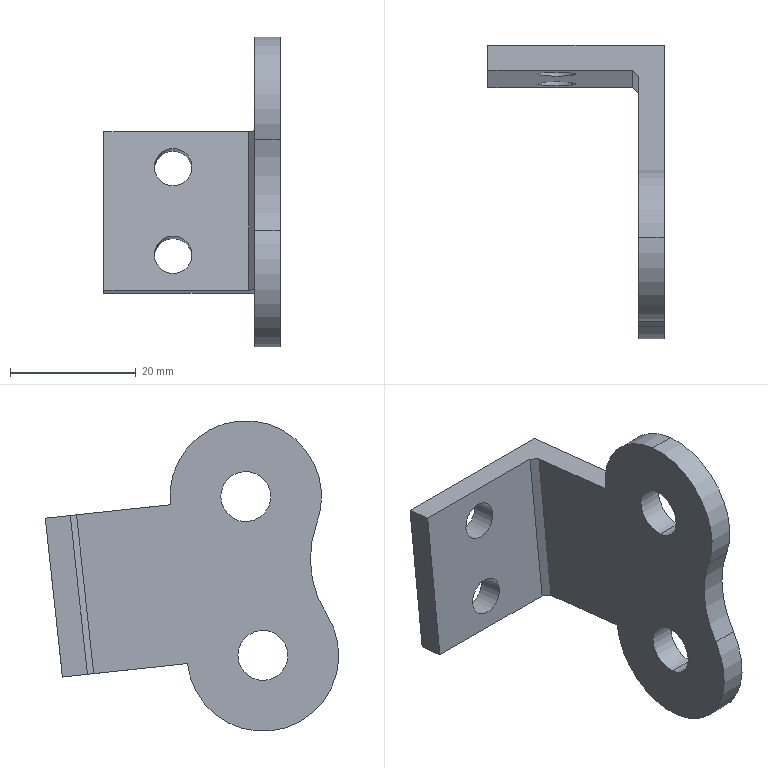Part | STEP file | Cut-Extrude 2-4 | 1 solid | 21 faces | box 28 x 46.671 x 49.383 mm | volume 7981 mm3 | cylinder 13 | plane 8 | commonest cylinder face diameters 6 x4 7.94 x4 24.13 x4 32.482 x1
STEP:
#1=CARTESIAN_POINT('',(303.74,-1270.259,3580.538));
#2=VERTEX_POINT('',#1);
#3=CARTESIAN_POINT('',(303.74,-1259.559,3567.248));
#4=VERTEX_POINT('',#3);
#5=CARTESIAN_POINT('',(303.74,-1271.554,3568.543));
#6=DIRECTION('',(-1.,0.,0.));
#7=DIRECTION('',(0.,0.1073,0.9942));
#8=AXIS2_PLACEMENT_3D('',#5,#6,#7);
#9=CIRCLE('',#8,12.065);
#10=EDGE_CURVE('',#2,#4,#9,.T.);
#11=ORIENTED_EDGE('',*,*,#10,.F.);
#12=CARTESIAN_POINT('',(307.74,-1270.259,3580.538));
#13=VERTEX_POINT('',#12);
#14=CARTESIAN_POINT('',(303.74,-1270.259,3580.538));
#15=DIRECTION('',(1.,0.,0.));
#16=VECTOR('',#15,1000.);
#17=LINE('',#14,#16);
#18=EDGE_CURVE('',#2,#13,#17,.T.);
#19=ORIENTED_EDGE('',*,*,#18,.T.);
#20=CARTESIAN_POINT('',(307.74,-1259.559,3567.248));
#21=VERTEX_POINT('',#20);
#22=CARTESIAN_POINT('',(307.74,-1271.554,3568.543));
#23=DIRECTION('',(-1.,0.,0.));
#24=DIRECTION('',(0.,0.1073,0.9942));
#25=AXIS2_PLACEMENT_3D('',#22,#23,#24);
#26=CIRCLE('',#25,12.065);
#27=EDGE_CURVE('',#13,#21,#26,.T.);
#28=ORIENTED_EDGE('',*,*,#27,.T.);
#29=CARTESIAN_POINT('',(303.74,-1259.559,3567.248));
#30=DIRECTION('',(1.,0.,0.));
#31=VECTOR('',#30,1000.);
#32=LINE('',#29,#31);
#33=EDGE_CURVE('',#4,#21,#32,.T.);
#34=ORIENTED_EDGE('',*,*,#33,.F.);
#35=EDGE_LOOP('',(#11,#19,#28,#34));
#36=FACE_OUTER_BOUND('',#35,.T.);
#37=CARTESIAN_POINT('',(303.74,-1271.554,3568.543));
#38=DIRECTION('',(1.,0.,0.));
#39=DIRECTION('',(0.,0.1073,0.9942));
#40=AXIS2_PLACEMENT_3D('',#37,#38,#39);
#41=CYLINDRICAL_SURFACE('',#40,12.065);
#42=ADVANCED_FACE('',(#36),#41,.T.);
#43=CARTESIAN_POINT('',(287.74,-1245.766,3545.944));
#44=VERTEX_POINT('',#43);
#45=CARTESIAN_POINT('',(293.74,-1245.766,3545.944));
#46=VERTEX_POINT('',#45);
#47=CARTESIAN_POINT('',(290.74,-1245.766,3545.944));
#48=DIRECTION('',(0.,-0.9942,0.1073));
#49=DIRECTION('',(1.,0.,0.));
#50=AXIS2_PLACEMENT_3D('',#47,#48,#49);
#51=CIRCLE('',#50,3.);
#52=EDGE_CURVE('',#44,#46,#51,.T.);
#53=ORIENTED_EDGE('',*,*,#52,.T.);
#54=CARTESIAN_POINT('',(293.74,-1241.789,3545.515));
#55=VERTEX_POINT('',#54);
#56=CARTESIAN_POINT('',(293.74,-1285.664,3550.251));
#57=DIRECTION('',(0.,0.9942,-0.1073));
#58=VECTOR('',#57,1000.);
#59=LINE('',#56,#58);
#60=EDGE_CURVE('',#46,#55,#59,.T.);
#61=ORIENTED_EDGE('',*,*,#60,.T.);
#62=CARTESIAN_POINT('',(287.74,-1241.789,3545.515));
#63=VERTEX_POINT('',#62);
#64=CARTESIAN_POINT('',(290.74,-1241.789,3545.515));
#65=DIRECTION('',(0.,0.9942,-0.1073));
#66=DIRECTION('',(-1.,0.,0.));
#67=AXIS2_PLACEMENT_3D('',#64,#65,#66);
#68=CIRCLE('',#67,3.);
#69=EDGE_CURVE('',#55,#63,#68,.T.);
#70=ORIENTED_EDGE('',*,*,#69,.T.);
#71=CARTESIAN_POINT('',(287.74,-1285.664,3550.251));
#72=DIRECTION('',(0.,0.9942,-0.1073));
#73=VECTOR('',#72,1000.);
#74=LINE('',#71,#73);
#75=EDGE_CURVE('',#44,#63,#74,.T.);
#76=ORIENTED_EDGE('',*,*,#75,.F.);
#77=EDGE_LOOP('',(#53,#61,#70,#76));
#78=FACE_OUTER_BOUND('',#77,.T.);
#79=CARTESIAN_POINT('',(290.74,-1285.664,3550.251));
#80=DIRECTION('',(0.,0.9942,-0.1073));
#81=DIRECTION('',(1.,0.,0.));
#82=AXIS2_PLACEMENT_3D('',#79,#80,#81);
#83=CYLINDRICAL_SURFACE('',#82,3.);
#84=ADVANCED_FACE('',(#78),#83,.F.);
#85=CARTESIAN_POINT('',(287.74,-1244.263,3559.863));
#86=VERTEX_POINT('',#85);
#87=CARTESIAN_POINT('',(293.74,-1244.263,3559.863));
#88=VERTEX_POINT('',#87);
#89=CARTESIAN_POINT('',(290.74,-1244.263,3559.863));
#90=DIRECTION('',(0.,-0.9942,0.1073));
#91=DIRECTION('',(1.,0.,0.));
#92=AXIS2_PLACEMENT_3D('',#89,#90,#91);
#93=CIRCLE('',#92,3.);
#94=EDGE_CURVE('',#86,#88,#93,.T.);
#95=ORIENTED_EDGE('',*,*,#94,.T.);
#96=CARTESIAN_POINT('',(293.74,-1240.286,3559.434));
#97=VERTEX_POINT('',#96);
#98=CARTESIAN_POINT('',(293.74,-1284.161,3564.171));
#99=DIRECTION('',(0.,0.9942,-0.1073));
#100=VECTOR('',#99,1000.);
#101=LINE('',#98,#100);
#102=EDGE_CURVE('',#88,#97,#101,.T.);
#103=ORIENTED_EDGE('',*,*,#102,.T.);
#104=CARTESIAN_POINT('',(287.74,-1240.286,3559.434));
#105=VERTEX_POINT('',#104);
#106=CARTESIAN_POINT('',(290.74,-1240.286,3559.434));
#107=DIRECTION('',(0.,0.9942,-0.1073));
#108=DIRECTION('',(1.,0.,0.));
#109=AXIS2_PLACEMENT_3D('',#106,#107,#108);
#110=CIRCLE('',#109,3.);
#111=EDGE_CURVE('',#97,#105,#110,.T.);
#112=ORIENTED_EDGE('',*,*,#111,.T.);
#113=CARTESIAN_POINT('',(287.74,-1284.161,3564.171));
#114=DIRECTION('',(0.,0.9942,-0.1073));
#115=VECTOR('',#114,1000.);
#116=LINE('',#113,#115);
#117=EDGE_CURVE('',#86,#105,#116,.T.);
#118=ORIENTED_EDGE('',*,*,#117,.F.);
#119=EDGE_LOOP('',(#95,#103,#112,#118));
#120=FACE_OUTER_BOUND('',#119,.T.);
#121=CARTESIAN_POINT('',(290.74,-1284.161,3564.171));
#122=DIRECTION('',(0.,0.9942,-0.1073));
#123=DIRECTION('',(1.,0.,0.));
#124=AXIS2_PLACEMENT_3D('',#121,#122,#123);
#125=CYLINDRICAL_SURFACE('',#124,3.);
#126=ADVANCED_FACE('',(#120),#125,.F.);
#127=CARTESIAN_POINT('',(303.74,-1271.128,3572.49));
#128=VERTEX_POINT('',#127);
#129=CARTESIAN_POINT('',(303.74,-1271.98,3564.596));
#130=VERTEX_POINT('',#129);
#131=CARTESIAN_POINT('',(303.74,-1271.554,3568.543));
#132=DIRECTION('',(1.,0.,0.));
#133=DIRECTION('',(0.,-0.1073,-0.9942));
#134=AXIS2_PLACEMENT_3D('',#131,#132,#133);
#135=CIRCLE('',#134,3.97);
#136=EDGE_CURVE('',#128,#130,#135,.T.);
#137=ORIENTED_EDGE('',*,*,#136,.F.);
#138=CARTESIAN_POINT('',(307.74,-1271.128,3572.49));
#139=VERTEX_POINT('',#138);
#140=CARTESIAN_POINT('',(303.74,-1271.128,3572.49));
#141=DIRECTION('',(-1.,0.,0.));
#142=VECTOR('',#141,1000.);
#143=LINE('',#140,#142);
#144=EDGE_CURVE('',#139,#128,#143,.T.);
#145=ORIENTED_EDGE('',*,*,#144,.F.);
#146=CARTESIAN_POINT('',(307.74,-1271.98,3564.596));
#147=VERTEX_POINT('',#146);
#148=CARTESIAN_POINT('',(307.74,-1271.554,3568.543));
#149=DIRECTION('',(1.,0.,0.));
#150=DIRECTION('',(0.,-0.1073,-0.9942));
#151=AXIS2_PLACEMENT_3D('',#148,#149,#150);
#152=CIRCLE('',#151,3.97);
#153=EDGE_CURVE('',#139,#147,#152,.T.);
#154=ORIENTED_EDGE('',*,*,#153,.T.);
#155=CARTESIAN_POINT('',(303.74,-1271.98,3564.596));
#156=DIRECTION('',(-1.,0.,0.));
#157=VECTOR('',#156,1000.);
#158=LINE('',#155,#157);
#159=EDGE_CURVE('',#147,#130,#158,.T.);
#160=ORIENTED_EDGE('',*,*,#159,.T.);
#161=EDGE_LOOP('',(#137,#145,#154,#160));
#162=FACE_OUTER_BOUND('',#161,.T.);
#163=CARTESIAN_POINT('',(303.74,-1271.554,3568.543));
#164=DIRECTION('',(1.,0.,0.));
#165=DIRECTION('',(0.,0.1073,0.9942));
#166=AXIS2_PLACEMENT_3D('',#163,#164,#165);
#167=CYLINDRICAL_SURFACE('',#166,3.97);
#168=ADVANCED_FACE('',(#162),#167,.F.);
#169=CARTESIAN_POINT('',(303.74,-1273.855,3547.236));
#170=VERTEX_POINT('',#169);
#171=CARTESIAN_POINT('',(303.74,-1274.707,3539.342));
#172=VERTEX_POINT('',#171);
#173=CARTESIAN_POINT('',(303.74,-1274.281,3543.289));
#174=DIRECTION('',(1.,0.,0.));
#175=DIRECTION('',(0.,0.1073,0.9942));
#176=AXIS2_PLACEMENT_3D('',#173,#174,#175);
#177=CIRCLE('',#176,3.97);
#178=EDGE_CURVE('',#170,#172,#177,.T.);
#179=ORIENTED_EDGE('',*,*,#178,.F.);
#180=CARTESIAN_POINT('',(307.74,-1273.855,3547.236));
#181=VERTEX_POINT('',#180);
#182=CARTESIAN_POINT('',(303.74,-1273.855,3547.236));
#183=DIRECTION('',(-1.,0.,0.));
#184=VECTOR('',#183,1000.);
#185=LINE('',#182,#184);
#186=EDGE_CURVE('',#181,#170,#185,.T.);
#187=ORIENTED_EDGE('',*,*,#186,.F.);
#188=CARTESIAN_POINT('',(307.74,-1274.707,3539.342));
#189=VERTEX_POINT('',#188);
#190=CARTESIAN_POINT('',(307.74,-1274.281,3543.289));
#191=DIRECTION('',(1.,0.,0.));
#192=DIRECTION('',(0.,0.1073,0.9942));
#193=AXIS2_PLACEMENT_3D('',#190,#191,#192);
#194=CIRCLE('',#193,3.97);
#195=EDGE_CURVE('',#181,#189,#194,.T.);
#196=ORIENTED_EDGE('',*,*,#195,.T.);
#197=CARTESIAN_POINT('',(303.74,-1274.707,3539.342));
#198=DIRECTION('',(-1.,0.,0.));
#199=VECTOR('',#198,1000.);
#200=LINE('',#197,#199);
#201=EDGE_CURVE('',#189,#172,#200,.T.);
#202=ORIENTED_EDGE('',*,*,#201,.T.);
#203=EDGE_LOOP('',(#179,#187,#196,#202));
#204=FACE_OUTER_BOUND('',#203,.T.);
#205=CARTESIAN_POINT('',(303.74,-1274.281,3543.289));
#206=DIRECTION('',(1.,0.,0.));
#207=DIRECTION('',(0.,0.1073,0.9942));
#208=AXIS2_PLACEMENT_3D('',#205,#206,#207);
#209=CYLINDRICAL_SURFACE('',#208,3.97);
#210=ADVANCED_FACE('',(#204),#209,.F.);
#211=CARTESIAN_POINT('',(303.74,-1275.576,3531.294));
#212=VERTEX_POINT('',#211);
#213=CARTESIAN_POINT('',(303.74,-1284.42,3549.829));
#214=VERTEX_POINT('',#213);
#215=CARTESIAN_POINT('',(303.74,-1274.281,3543.289));
#216=DIRECTION('',(-1.,0.,0.));
#217=DIRECTION('',(0.,0.1073,0.9942));
#218=AXIS2_PLACEMENT_3D('',#215,#216,#217);
#219=CIRCLE('',#218,12.065);
#220=EDGE_CURVE('',#212,#214,#219,.T.);
#221=ORIENTED_EDGE('',*,*,#220,.F.);
#222=CARTESIAN_POINT('',(307.74,-1275.576,3531.294));
#223=VERTEX_POINT('',#222);
#224=CARTESIAN_POINT('',(303.74,-1275.576,3531.294));
#225=DIRECTION('',(1.,0.,0.));
#226=VECTOR('',#225,1000.);
#227=LINE('',#224,#226);
#228=EDGE_CURVE('',#212,#223,#227,.T.);
#229=ORIENTED_EDGE('',*,*,#228,.T.);
#230=CARTESIAN_POINT('',(307.74,-1284.42,3549.829));
#231=VERTEX_POINT('',#230);
#232=CARTESIAN_POINT('',(307.74,-1274.281,3543.289));
#233=DIRECTION('',(-1.,0.,0.));
#234=DIRECTION('',(0.,0.1073,0.9942));
#235=AXIS2_PLACEMENT_3D('',#232,#233,#234);
#236=CIRCLE('',#235,12.065);
#237=EDGE_CURVE('',#223,#231,#236,.T.);
#238=ORIENTED_EDGE('',*,*,#237,.T.);
#239=CARTESIAN_POINT('',(303.74,-1284.42,3549.829));
#240=DIRECTION('',(1.,0.,0.));
#241=VECTOR('',#240,1000.);
#242=LINE('',#239,#241);
#243=EDGE_CURVE('',#214,#231,#242,.T.);
#244=ORIENTED_EDGE('',*,*,#243,.F.);
#245=EDGE_LOOP('',(#221,#229,#238,#244));
#246=FACE_OUTER_BOUND('',#245,.T.);
#247=CARTESIAN_POINT('',(303.74,-1274.281,3543.289));
#248=DIRECTION('',(1.,0.,0.));
#249=DIRECTION('',(0.,0.1073,0.9942));
#250=AXIS2_PLACEMENT_3D('',#247,#248,#249);
#251=CYLINDRICAL_SURFACE('',#250,12.065);
#252=ADVANCED_FACE('',(#246),#251,.T.);
#253=CARTESIAN_POINT('',(303.74,-1271.554,3568.543));
#254=DIRECTION('',(1.,0.,0.));
#255=DIRECTION('',(0.,-0.1073,-0.9942));
#256=AXIS2_PLACEMENT_3D('',#253,#254,#255);
#257=CIRCLE('',#256,3.97);
#258=EDGE_CURVE('',#130,#128,#257,.T.);
#259=ORIENTED_EDGE('',*,*,#258,.T.);
#260=ORIENTED_EDGE('',*,*,#136,.T.);
#261=EDGE_LOOP('',(#259,#260));
#262=FACE_BOUND('',#261,.T.);
#263=CARTESIAN_POINT('',(303.74,-1274.281,3543.289));
#264=DIRECTION('',(1.,0.,0.));
#265=DIRECTION('',(0.,0.1073,0.9942));
#266=AXIS2_PLACEMENT_3D('',#263,#264,#265);
#267=CIRCLE('',#266,3.97);
#268=EDGE_CURVE('',#172,#170,#267,.T.);
#269=ORIENTED_EDGE('',*,*,#268,.T.);
#270=ORIENTED_EDGE('',*,*,#178,.T.);
#271=EDGE_LOOP('',(#269,#270));
#272=FACE_BOUND('',#271,.T.);
#273=CARTESIAN_POINT('',(303.74,-1244.646,3565.637));
#274=VERTEX_POINT('',#273);
#275=CARTESIAN_POINT('',(303.74,-1239.674,3565.101));
#276=DIRECTION('',(0.,0.9942,-0.1073));
#277=VECTOR('',#276,1000.);
#278=LINE('',#275,#277);
#279=EDGE_CURVE('',#4,#274,#278,.T.);
#280=ORIENTED_EDGE('',*,*,#279,.T.);
#281=CARTESIAN_POINT('',(303.74,-1247.372,3540.384));
#282=VERTEX_POINT('',#281);
#283=CARTESIAN_POINT('',(303.74,-1247.372,3540.384));
#284=DIRECTION('',(0.,-0.1073,-0.9942));
#285=VECTOR('',#284,1000.);
#286=LINE('',#283,#285);
#287=EDGE_CURVE('',#274,#282,#286,.T.);
#288=ORIENTED_EDGE('',*,*,#287,.T.);
#289=CARTESIAN_POINT('',(303.74,-1262.285,3541.994));
#290=VERTEX_POINT('',#289);
#291=CARTESIAN_POINT('',(303.74,-1262.285,3541.994));
#292=DIRECTION('',(0.,-0.9942,0.1073));
#293=VECTOR('',#292,1000.);
#294=LINE('',#291,#293);
#295=EDGE_CURVE('',#282,#290,#294,.T.);
#296=ORIENTED_EDGE('',*,*,#295,.T.);
#297=CARTESIAN_POINT('',(303.74,-1274.281,3543.289));
#298=DIRECTION('',(-1.,0.,0.));
#299=DIRECTION('',(0.,0.1073,0.9942));
#300=AXIS2_PLACEMENT_3D('',#297,#298,#299);
#301=CIRCLE('',#300,12.065);
#302=EDGE_CURVE('',#290,#212,#301,.T.);
#303=ORIENTED_EDGE('',*,*,#302,.T.);
#304=ORIENTED_EDGE('',*,*,#220,.T.);
#305=CARTESIAN_POINT('',(303.74,-1282.855,3564.318));
#306=VERTEX_POINT('',#305);
#307=CARTESIAN_POINT('',(303.74,-1298.069,3558.631));
#308=DIRECTION('',(1.,0.,0.));
#309=DIRECTION('',(0.,0.1073,0.9942));
#310=AXIS2_PLACEMENT_3D('',#307,#308,#309);
#311=CIRCLE('',#310,16.241);
#312=EDGE_CURVE('',#214,#306,#311,.T.);
#313=ORIENTED_EDGE('',*,*,#312,.T.);
#314=CARTESIAN_POINT('',(303.74,-1271.554,3568.543));
#315=DIRECTION('',(-1.,0.,0.));
#316=DIRECTION('',(0.,0.1073,0.9942));
#317=AXIS2_PLACEMENT_3D('',#314,#315,#316);
#318=CIRCLE('',#317,12.065);
#319=EDGE_CURVE('',#306,#2,#318,.T.);
#320=ORIENTED_EDGE('',*,*,#319,.T.);
#321=ORIENTED_EDGE('',*,*,#10,.T.);
#322=EDGE_LOOP('',(#280,#288,#296,#303,#304,#313,#320,#321));
#323=FACE_OUTER_BOUND('',#322,.T.);
#324=CARTESIAN_POINT('',(303.74,-1274.281,3543.289));
#325=DIRECTION('',(-1.,0.,0.));
#326=DIRECTION('',(0.,-0.1073,-0.9942));
#327=AXIS2_PLACEMENT_3D('',#324,#325,#326);
#328=PLANE('',#327);
#329=ADVANCED_FACE('',(#262,#272,#323),#328,.T.);
#330=ORIENTED_EDGE('',*,*,#228,.F.);
#331=ORIENTED_EDGE('',*,*,#302,.F.);
#332=CARTESIAN_POINT('',(307.74,-1262.285,3541.994));
#333=VERTEX_POINT('',#332);
#334=CARTESIAN_POINT('',(303.74,-1262.285,3541.994));
#335=DIRECTION('',(1.,0.,0.));
#336=VECTOR('',#335,1000.);
#337=LINE('',#334,#336);
#338=EDGE_CURVE('',#290,#333,#337,.T.);
#339=ORIENTED_EDGE('',*,*,#338,.T.);
#340=CARTESIAN_POINT('',(307.74,-1274.281,3543.289));
#341=DIRECTION('',(-1.,0.,0.));
#342=DIRECTION('',(0.,0.1073,0.9942));
#343=AXIS2_PLACEMENT_3D('',#340,#341,#342);
#344=CIRCLE('',#343,12.065);
#345=EDGE_CURVE('',#333,#223,#344,.T.);
#346=ORIENTED_EDGE('',*,*,#345,.T.);
#347=EDGE_LOOP('',(#330,#331,#339,#346));
#348=FACE_OUTER_BOUND('',#347,.T.);
#349=CARTESIAN_POINT('',(303.74,-1274.281,3543.289));
#350=DIRECTION('',(1.,0.,0.));
#351=DIRECTION('',(0.,0.1073,0.9942));
#352=AXIS2_PLACEMENT_3D('',#349,#350,#351);
#353=CYLINDRICAL_SURFACE('',#352,12.065);
#354=ADVANCED_FACE('',(#348),#353,.T.);
#355=CARTESIAN_POINT('',(307.74,-1282.855,3564.318));
#356=VERTEX_POINT('',#355);
#357=CARTESIAN_POINT('',(307.74,-1298.069,3558.631));
#358=DIRECTION('',(1.,0.,0.));
#359=DIRECTION('',(0.,0.1073,0.9942));
#360=AXIS2_PLACEMENT_3D('',#357,#358,#359);
#361=CIRCLE('',#360,16.241);
#362=EDGE_CURVE('',#231,#356,#361,.T.);
#363=ORIENTED_EDGE('',*,*,#362,.T.);
#364=CARTESIAN_POINT('',(303.74,-1282.855,3564.318));
#365=DIRECTION('',(1.,0.,0.));
#366=VECTOR('',#365,1000.);
#367=LINE('',#364,#366);
#368=EDGE_CURVE('',#306,#356,#367,.T.);
#369=ORIENTED_EDGE('',*,*,#368,.F.);
#370=ORIENTED_EDGE('',*,*,#312,.F.);
#371=ORIENTED_EDGE('',*,*,#243,.T.);
#372=EDGE_LOOP('',(#363,#369,#370,#371));
#373=FACE_OUTER_BOUND('',#372,.T.);
#374=CARTESIAN_POINT('',(303.74,-1298.069,3558.631));
#375=DIRECTION('',(1.,0.,0.));
#376=DIRECTION('',(0.,0.1073,0.9942));
#377=AXIS2_PLACEMENT_3D('',#374,#375,#376);
#378=CYLINDRICAL_SURFACE('',#377,16.241);
#379=ADVANCED_FACE('',(#373),#378,.F.);
#380=ORIENTED_EDGE('',*,*,#18,.F.);
#381=ORIENTED_EDGE('',*,*,#319,.F.);
#382=ORIENTED_EDGE('',*,*,#368,.T.);
#383=CARTESIAN_POINT('',(307.74,-1271.554,3568.543));
#384=DIRECTION('',(-1.,0.,0.));
#385=DIRECTION('',(0.,0.1073,0.9942));
#386=AXIS2_PLACEMENT_3D('',#383,#384,#385);
#387=CIRCLE('',#386,12.065);
#388=EDGE_CURVE('',#356,#13,#387,.T.);
#389=ORIENTED_EDGE('',*,*,#388,.T.);
#390=EDGE_LOOP('',(#380,#381,#382,#389));
#391=FACE_OUTER_BOUND('',#390,.T.);
#392=CARTESIAN_POINT('',(303.74,-1271.554,3568.543));
#393=DIRECTION('',(1.,0.,0.));
#394=DIRECTION('',(0.,0.1073,0.9942));
#395=AXIS2_PLACEMENT_3D('',#392,#393,#394);
#396=CYLINDRICAL_SURFACE('',#395,12.065);
#397=ADVANCED_FACE('',(#391),#396,.T.);
#398=CARTESIAN_POINT('',(307.74,-1239.674,3565.101));
#399=VERTEX_POINT('',#398);
#400=CARTESIAN_POINT('',(307.74,-1239.674,3565.101));
#401=DIRECTION('',(0.,0.9942,-0.1073));
#402=VECTOR('',#401,1000.);
#403=LINE('',#400,#402);
#404=EDGE_CURVE('',#21,#399,#403,.T.);
#405=ORIENTED_EDGE('',*,*,#404,.T.);
#406=CARTESIAN_POINT('',(279.74,-1239.674,3565.101));
#407=VERTEX_POINT('',#406);
#408=CARTESIAN_POINT('',(303.74,-1239.674,3565.101));
#409=DIRECTION('',(1.,0.,0.));
#410=VECTOR('',#409,1000.);
#411=LINE('',#408,#410);
#412=EDGE_CURVE('',#407,#399,#411,.T.);
#413=ORIENTED_EDGE('',*,*,#412,.F.);
#414=CARTESIAN_POINT('',(279.74,-1243.651,3565.53));
#415=VERTEX_POINT('',#414);
#416=CARTESIAN_POINT('',(279.74,-1243.651,3565.53));
#417=DIRECTION('',(0.,0.9942,-0.1073));
#418=VECTOR('',#417,1000.);
#419=LINE('',#416,#418);
#420=EDGE_CURVE('',#415,#407,#419,.T.);
#421=ORIENTED_EDGE('',*,*,#420,.F.);
#422=CARTESIAN_POINT('',(302.74,-1243.651,3565.53));
#423=VERTEX_POINT('',#422);
#424=CARTESIAN_POINT('',(303.74,-1243.651,3565.53));
#425=DIRECTION('',(1.,0.,0.));
#426=VECTOR('',#425,1000.);
#427=LINE('',#424,#426);
#428=EDGE_CURVE('',#415,#423,#427,.T.);
#429=ORIENTED_EDGE('',*,*,#428,.T.);
#430=CARTESIAN_POINT('',(301.24,-1242.16,3565.369));
#431=DIRECTION('',(0.7071,-0.703,0.0759));
#432=VECTOR('',#431,1000.);
#433=LINE('',#430,#432);
#434=EDGE_CURVE('',#423,#274,#433,.T.);
#435=ORIENTED_EDGE('',*,*,#434,.T.);
#436=ORIENTED_EDGE('',*,*,#279,.F.);
#437=ORIENTED_EDGE('',*,*,#33,.T.);
#438=EDGE_LOOP('',(#405,#413,#421,#429,#435,#436,#437));
#439=FACE_OUTER_BOUND('',#438,.T.);
#440=CARTESIAN_POINT('',(303.74,-1239.674,3565.101));
#441=DIRECTION('',(0.,-0.1073,-0.9942));
#442=DIRECTION('',(0.,0.9942,-0.1073));
#443=AXIS2_PLACEMENT_3D('',#440,#441,#442);
#444=PLANE('',#443);
#445=ADVANCED_FACE('',(#439),#444,.F.);
#446=CARTESIAN_POINT('',(290.74,-1241.789,3545.515));
#447=DIRECTION('',(0.,0.9942,-0.1073));
#448=DIRECTION('',(-1.,0.,0.));
#449=AXIS2_PLACEMENT_3D('',#446,#447,#448);
#450=CIRCLE('',#449,3.);
#451=EDGE_CURVE('',#63,#55,#450,.T.);
#452=ORIENTED_EDGE('',*,*,#451,.F.);
#453=ORIENTED_EDGE('',*,*,#69,.F.);
#454=EDGE_LOOP('',(#452,#453));
#455=FACE_BOUND('',#454,.T.);
#456=CARTESIAN_POINT('',(290.74,-1240.286,3559.434));
#457=DIRECTION('',(0.,0.9942,-0.1073));
#458=DIRECTION('',(1.,0.,0.));
#459=AXIS2_PLACEMENT_3D('',#456,#457,#458);
#460=CIRCLE('',#459,3.);
#461=EDGE_CURVE('',#105,#97,#460,.T.);
#462=ORIENTED_EDGE('',*,*,#461,.F.);
#463=ORIENTED_EDGE('',*,*,#111,.F.);
#464=EDGE_LOOP('',(#462,#463));
#465=FACE_BOUND('',#464,.T.);
#466=CARTESIAN_POINT('',(307.74,-1242.401,3539.847));
#467=VERTEX_POINT('',#466);
#468=CARTESIAN_POINT('',(307.74,-1242.401,3539.847));
#469=DIRECTION('',(0.,-0.1073,-0.9942));
#470=VECTOR('',#469,1000.);
#471=LINE('',#468,#470);
#472=EDGE_CURVE('',#399,#467,#471,.T.);
#473=ORIENTED_EDGE('',*,*,#472,.T.);
#474=CARTESIAN_POINT('',(279.74,-1242.401,3539.847));
#475=VERTEX_POINT('',#474);
#476=CARTESIAN_POINT('',(303.74,-1242.401,3539.847));
#477=DIRECTION('',(1.,0.,0.));
#478=VECTOR('',#477,1000.);
#479=LINE('',#476,#478);
#480=EDGE_CURVE('',#475,#467,#479,.T.);
#481=ORIENTED_EDGE('',*,*,#480,.F.);
#482=CARTESIAN_POINT('',(279.74,-1242.401,3539.847));
#483=DIRECTION('',(0.,0.1073,0.9942));
#484=VECTOR('',#483,1000.);
#485=LINE('',#482,#484);
#486=EDGE_CURVE('',#475,#407,#485,.T.);
#487=ORIENTED_EDGE('',*,*,#486,.T.);
#488=ORIENTED_EDGE('',*,*,#412,.T.);
#489=EDGE_LOOP('',(#473,#481,#487,#488));
#490=FACE_OUTER_BOUND('',#489,.T.);
#491=CARTESIAN_POINT('',(303.74,-1242.401,3539.847));
#492=DIRECTION('',(0.,-0.9942,0.1073));
#493=DIRECTION('',(-1.,0.,0.));
#494=AXIS2_PLACEMENT_3D('',#491,#492,#493);
#495=PLANE('',#494);
#496=ADVANCED_FACE('',(#455,#465,#490),#495,.F.);
#497=CARTESIAN_POINT('',(307.74,-1262.285,3541.994));
#498=DIRECTION('',(0.,-0.9942,0.1073));
#499=VECTOR('',#498,1000.);
#500=LINE('',#497,#499);
#501=EDGE_CURVE('',#467,#333,#500,.T.);
#502=ORIENTED_EDGE('',*,*,#501,.T.);
#503=ORIENTED_EDGE('',*,*,#338,.F.);
#504=ORIENTED_EDGE('',*,*,#295,.F.);
#505=CARTESIAN_POINT('',(302.74,-1246.378,3540.277));
#506=VERTEX_POINT('',#505);
#507=CARTESIAN_POINT('',(311.24,-1254.829,3541.189));
#508=DIRECTION('',(-0.7071,0.703,-0.0759));
#509=VECTOR('',#508,1000.);
#510=LINE('',#507,#509);
#511=EDGE_CURVE('',#282,#506,#510,.T.);
#512=ORIENTED_EDGE('',*,*,#511,.T.);
#513=CARTESIAN_POINT('',(279.74,-1246.378,3540.277));
#514=VERTEX_POINT('',#513);
#515=CARTESIAN_POINT('',(303.74,-1246.378,3540.277));
#516=DIRECTION('',(-1.,0.,0.));
#517=VECTOR('',#516,1000.);
#518=LINE('',#515,#517);
#519=EDGE_CURVE('',#506,#514,#518,.T.);
#520=ORIENTED_EDGE('',*,*,#519,.T.);
#521=CARTESIAN_POINT('',(279.74,-1246.378,3540.277));
#522=DIRECTION('',(0.,0.9942,-0.1073));
#523=VECTOR('',#522,1000.);
#524=LINE('',#521,#523);
#525=EDGE_CURVE('',#514,#475,#524,.T.);
#526=ORIENTED_EDGE('',*,*,#525,.T.);
#527=ORIENTED_EDGE('',*,*,#480,.T.);
#528=EDGE_LOOP('',(#502,#503,#504,#512,#520,#526,#527));
#529=FACE_OUTER_BOUND('',#528,.T.);
#530=CARTESIAN_POINT('',(303.74,-1262.285,3541.994));
#531=DIRECTION('',(0.,0.1073,0.9942));
#532=DIRECTION('',(0.,-0.9942,0.1073));
#533=AXIS2_PLACEMENT_3D('',#530,#531,#532);
#534=PLANE('',#533);
#535=ADVANCED_FACE('',(#529),#534,.F.);
#536=CARTESIAN_POINT('',(307.74,-1271.554,3568.543));
#537=DIRECTION('',(1.,0.,0.));
#538=DIRECTION('',(0.,-0.1073,-0.9942));
#539=AXIS2_PLACEMENT_3D('',#536,#537,#538);
#540=CIRCLE('',#539,3.97);
#541=EDGE_CURVE('',#147,#139,#540,.T.);
#542=ORIENTED_EDGE('',*,*,#541,.F.);
#543=ORIENTED_EDGE('',*,*,#153,.F.);
#544=EDGE_LOOP('',(#542,#543));
#545=FACE_BOUND('',#544,.T.);
#546=CARTESIAN_POINT('',(307.74,-1274.281,3543.289));
#547=DIRECTION('',(1.,0.,0.));
#548=DIRECTION('',(0.,0.1073,0.9942));
#549=AXIS2_PLACEMENT_3D('',#546,#547,#548);
#550=CIRCLE('',#549,3.97);
#551=EDGE_CURVE('',#189,#181,#550,.T.);
#552=ORIENTED_EDGE('',*,*,#551,.F.);
#553=ORIENTED_EDGE('',*,*,#195,.F.);
#554=EDGE_LOOP('',(#552,#553));
#555=FACE_BOUND('',#554,.T.);
#556=ORIENTED_EDGE('',*,*,#345,.F.);
#557=ORIENTED_EDGE('',*,*,#501,.F.);
#558=ORIENTED_EDGE('',*,*,#472,.F.);
#559=ORIENTED_EDGE('',*,*,#404,.F.);
#560=ORIENTED_EDGE('',*,*,#27,.F.);
#561=ORIENTED_EDGE('',*,*,#388,.F.);
#562=ORIENTED_EDGE('',*,*,#362,.F.);
#563=ORIENTED_EDGE('',*,*,#237,.F.);
#564=EDGE_LOOP('',(#556,#557,#558,#559,#560,#561,#562,#563));
#565=FACE_OUTER_BOUND('',#564,.T.);
#566=CARTESIAN_POINT('',(307.74,-1274.281,3543.289));
#567=DIRECTION('',(-1.,0.,0.));
#568=DIRECTION('',(0.,-0.1073,-0.9942));
#569=AXIS2_PLACEMENT_3D('',#566,#567,#568);
#570=PLANE('',#569);
#571=ADVANCED_FACE('',(#545,#555,#565),#570,.F.);
#572=ORIENTED_EDGE('',*,*,#186,.T.);
#573=ORIENTED_EDGE('',*,*,#268,.F.);
#574=ORIENTED_EDGE('',*,*,#201,.F.);
#575=ORIENTED_EDGE('',*,*,#551,.T.);
#576=EDGE_LOOP('',(#572,#573,#574,#575));
#577=FACE_OUTER_BOUND('',#576,.T.);
#578=CARTESIAN_POINT('',(303.74,-1274.281,3543.289));
#579=DIRECTION('',(1.,0.,0.));
#580=DIRECTION('',(0.,0.1073,0.9942));
#581=AXIS2_PLACEMENT_3D('',#578,#579,#580);
#582=CYLINDRICAL_SURFACE('',#581,3.97);
#583=ADVANCED_FACE('',(#577),#582,.F.);
#584=ORIENTED_EDGE('',*,*,#144,.T.);
#585=ORIENTED_EDGE('',*,*,#258,.F.);
#586=ORIENTED_EDGE('',*,*,#159,.F.);
#587=ORIENTED_EDGE('',*,*,#541,.T.);
#588=EDGE_LOOP('',(#584,#585,#586,#587));
#589=FACE_OUTER_BOUND('',#588,.T.);
#590=CARTESIAN_POINT('',(303.74,-1271.554,3568.543));
#591=DIRECTION('',(1.,0.,0.));
#592=DIRECTION('',(0.,0.1073,0.9942));
#593=AXIS2_PLACEMENT_3D('',#590,#591,#592);
#594=CYLINDRICAL_SURFACE('',#593,3.97);
#595=ADVANCED_FACE('',(#589),#594,.F.);
#596=ORIENTED_EDGE('',*,*,#486,.F.);
#597=ORIENTED_EDGE('',*,*,#525,.F.);
#598=CARTESIAN_POINT('',(279.74,-1246.378,3540.277));
#599=DIRECTION('',(0.,0.1073,0.9942));
#600=VECTOR('',#599,1000.);
#601=LINE('',#598,#600);
#602=EDGE_CURVE('',#514,#415,#601,.T.);
#603=ORIENTED_EDGE('',*,*,#602,.T.);
#604=ORIENTED_EDGE('',*,*,#420,.T.);
#605=EDGE_LOOP('',(#596,#597,#603,#604));
#606=FACE_OUTER_BOUND('',#605,.T.);
#607=CARTESIAN_POINT('',(279.74,-1246.378,3540.277));
#608=DIRECTION('',(-1.,0.,0.));
#609=DIRECTION('',(0.,-0.1073,-0.9942));
#610=AXIS2_PLACEMENT_3D('',#607,#608,#609);
#611=PLANE('',#610);
#612=ADVANCED_FACE('',(#606),#611,.T.);
#613=ORIENTED_EDGE('',*,*,#52,.F.);
#614=CARTESIAN_POINT('',(290.74,-1245.766,3545.944));
#615=DIRECTION('',(0.,-0.9942,0.1073));
#616=DIRECTION('',(1.,0.,0.));
#617=AXIS2_PLACEMENT_3D('',#614,#615,#616);
#618=CIRCLE('',#617,3.);
#619=EDGE_CURVE('',#46,#44,#618,.T.);
#620=ORIENTED_EDGE('',*,*,#619,.F.);
#621=EDGE_LOOP('',(#613,#620));
#622=FACE_BOUND('',#621,.T.);
#623=ORIENTED_EDGE('',*,*,#94,.F.);
#624=CARTESIAN_POINT('',(290.74,-1244.263,3559.863));
#625=DIRECTION('',(0.,-0.9942,0.1073));
#626=DIRECTION('',(1.,0.,0.));
#627=AXIS2_PLACEMENT_3D('',#624,#625,#626);
#628=CIRCLE('',#627,3.);
#629=EDGE_CURVE('',#88,#86,#628,.T.);
#630=ORIENTED_EDGE('',*,*,#629,.F.);
#631=EDGE_LOOP('',(#623,#630));
#632=FACE_BOUND('',#631,.T.);
#633=ORIENTED_EDGE('',*,*,#519,.F.);
#634=CARTESIAN_POINT('',(302.74,-1243.651,3565.53));
#635=DIRECTION('',(0.,0.1073,0.9942));
#636=VECTOR('',#635,1000.);
#637=LINE('',#634,#636);
#638=EDGE_CURVE('',#506,#423,#637,.T.);
#639=ORIENTED_EDGE('',*,*,#638,.T.);
#640=ORIENTED_EDGE('',*,*,#428,.F.);
#641=ORIENTED_EDGE('',*,*,#602,.F.);
#642=EDGE_LOOP('',(#633,#639,#640,#641));
#643=FACE_OUTER_BOUND('',#642,.T.);
#644=CARTESIAN_POINT('',(307.74,-1242.322,3577.845));
#645=DIRECTION('',(0.,-0.9942,0.1073));
#646=DIRECTION('',(-1.,0.,0.));
#647=AXIS2_PLACEMENT_3D('',#644,#645,#646);
#648=PLANE('',#647);
#649=ADVANCED_FACE('',(#622,#632,#643),#648,.T.);
#650=ORIENTED_EDGE('',*,*,#434,.F.);
#651=ORIENTED_EDGE('',*,*,#638,.F.);
#652=ORIENTED_EDGE('',*,*,#511,.F.);
#653=ORIENTED_EDGE('',*,*,#287,.F.);
#654=EDGE_LOOP('',(#650,#651,#652,#653));
#655=FACE_OUTER_BOUND('',#654,.T.);
#656=CARTESIAN_POINT('',(303.74,-1247.372,3540.384));
#657=DIRECTION('',(-0.7071,-0.703,0.0759));
#658=DIRECTION('',(0.,-0.1073,-0.9942));
#659=AXIS2_PLACEMENT_3D('',#656,#657,#658);
#660=PLANE('',#659);
#661=ADVANCED_FACE('',(#655),#660,.T.);
#662=ORIENTED_EDGE('',*,*,#102,.F.);
#663=ORIENTED_EDGE('',*,*,#629,.T.);
#664=ORIENTED_EDGE('',*,*,#117,.T.);
#665=ORIENTED_EDGE('',*,*,#461,.T.);
#666=EDGE_LOOP('',(#662,#663,#664,#665));
#667=FACE_OUTER_BOUND('',#666,.T.);
#668=CARTESIAN_POINT('',(290.74,-1284.161,3564.171));
#669=DIRECTION('',(0.,0.9942,-0.1073));
#670=DIRECTION('',(1.,0.,0.));
#671=AXIS2_PLACEMENT_3D('',#668,#669,#670);
#672=CYLINDRICAL_SURFACE('',#671,3.);
#673=ADVANCED_FACE('',(#667),#672,.F.);
#674=ORIENTED_EDGE('',*,*,#60,.F.);
#675=ORIENTED_EDGE('',*,*,#619,.T.);
#676=ORIENTED_EDGE('',*,*,#75,.T.);
#677=ORIENTED_EDGE('',*,*,#451,.T.);
#678=EDGE_LOOP('',(#674,#675,#676,#677));
#679=FACE_OUTER_BOUND('',#678,.T.);
#680=CARTESIAN_POINT('',(290.74,-1285.664,3550.251));
#681=DIRECTION('',(0.,0.9942,-0.1073));
#682=DIRECTION('',(1.,0.,0.));
#683=AXIS2_PLACEMENT_3D('',#680,#681,#682);
#684=CYLINDRICAL_SURFACE('',#683,3.);
#685=ADVANCED_FACE('',(#679),#684,.F.);
#686=CLOSED_SHELL('',(#42,#84,#126,#168,#210,#252,#329,#354,#379,#397,#445,#496,#535,#571,#583,#595,#612,#649,#661,#673,#685));
#687=MANIFOLD_SOLID_BREP('',#686);
#688=CARTESIAN_POINT('',(0.,0.,0.));
#689=DIRECTION('',(0.,0.,1.));
#690=DIRECTION('',(1.,0.,0.));
#691=AXIS2_PLACEMENT_3D('',#688,#689,#690);
#692=(LENGTH_UNIT()NAMED_UNIT(*)SI_UNIT(.MILLI.,.METRE.));
#693=UNCERTAINTY_MEASURE_WITH_UNIT(LENGTH_MEASURE(0.00001),#692,'','');
#694=(NAMED_UNIT(*)PLANE_ANGLE_UNIT()SI_UNIT($,.RADIAN.));
#695=(NAMED_UNIT(*)SI_UNIT($,.STERADIAN.)SOLID_ANGLE_UNIT());
#696=(GEOMETRIC_REPRESENTATION_CONTEXT(3)GLOBAL_UNCERTAINTY_ASSIGNED_CONTEXT((#693))GLOBAL_UNIT_ASSIGNED_CONTEXT((#692,#694,#695))REPRESENTATION_CONTEXT('',''));
#697=ADVANCED_BREP_SHAPE_REPRESENTATION('',(#687,#691),#696);